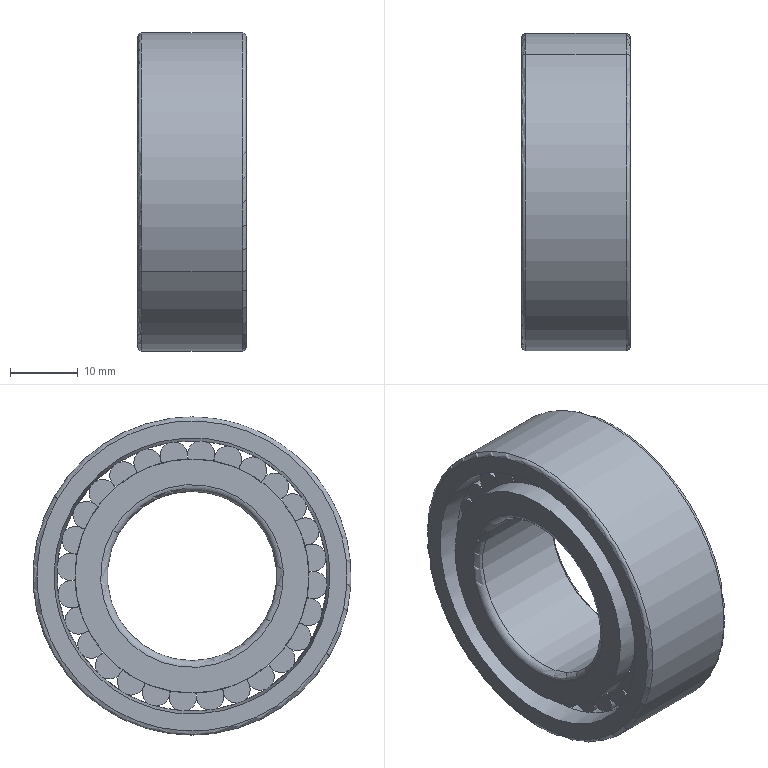Part | NX | features BREP 1 | 1 solid | 264 faces | box 16 x 47 x 47 mm | volume 16008 mm3 | cylinder 128 | plane 120 | torus 12 | cone 4 | commonest cylinder face diameters 4.02 x112 34.56 x6 31.978 x4 25 x2 40 x2 47 x2